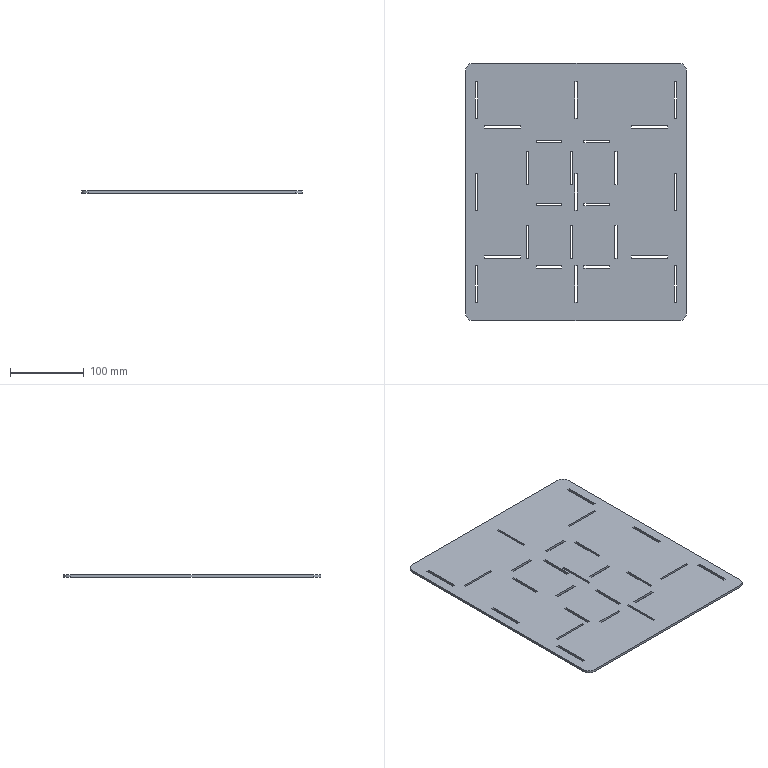Part | SolidWorks | features FlatPattern 1, SMBaseFlange 1, SheetMetal 1 | 1 solid | 110 faces | box 300 x 350 x 3.2 mm | volume 324154 mm3 | plane 106 | cylinder 4 | commonest cylinder face diameters 20 x4